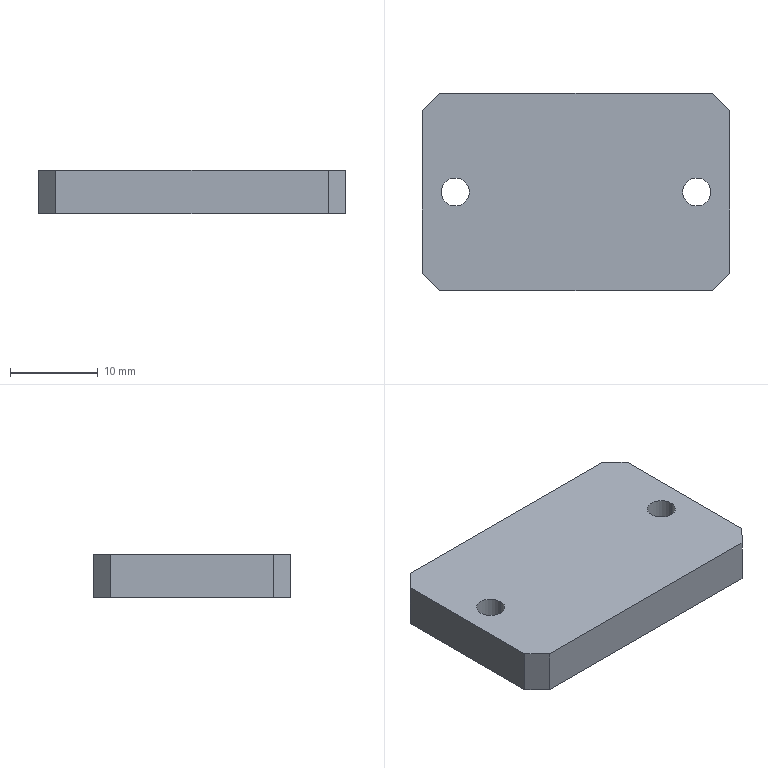Part | STEP file | PN_0031 | 1 solid | 14 faces | box 35 x 22.5 x 5 mm | volume 3817 mm3 | plane 10 | cylinder 4 | commonest cylinder face diameters 3.2 x4
STEP:
#1=CARTESIAN_POINT('',(0.,0.,0.));
#2=DIRECTION('',(0.,0.,1.));
#3=DIRECTION('',(1.,0.,0.));
#4=AXIS2_PLACEMENT_3D('',#1,#2,#3);
#5=CARTESIAN_POINT('',(-12.15,0.,0.));
#6=VERTEX_POINT('',#5);
#7=CARTESIAN_POINT('',(-12.15,0.,5.));
#8=VERTEX_POINT('',#7);
#9=CARTESIAN_POINT('',(-12.15,0.,5.));
#10=DIRECTION('',(0.,0.,1.));
#11=VECTOR('',#10,1.);
#12=LINE('',#9,#11);
#13=CARTESIAN_POINT('',(-13.75,0.,5.));
#14=DIRECTION('',(0.,0.,1.));
#15=DIRECTION('',(1.,0.,0.));
#16=AXIS2_PLACEMENT_3D('',#13,#14,#15);
#17=CYLINDRICAL_SURFACE('',#16,1.6);
#18=CARTESIAN_POINT('',(6.283,0.));
#19=DIRECTION('',(0.,1.));
#20=VECTOR('',#19,1.);
#21=LINE('',#18,#20);
#22=(GEOMETRIC_REPRESENTATION_CONTEXT(2)PARAMETRIC_REPRESENTATION_CONTEXT()REPRESENTATION_CONTEXT('',''));
#23=DEFINITIONAL_REPRESENTATION('',(#21),#22);
#24=PCURVE('',#17,#23);
#25=CARTESIAN_POINT('',(-13.75,0.,5.));
#26=DIRECTION('',(0.,0.,1.));
#27=DIRECTION('',(1.,0.,0.));
#28=AXIS2_PLACEMENT_3D('',#25,#26,#27);
#29=CYLINDRICAL_SURFACE('',#28,1.6);
#30=CARTESIAN_POINT('',(0.,0.));
#31=DIRECTION('',(0.,1.));
#32=VECTOR('',#31,1.);
#33=LINE('',#30,#32);
#34=(GEOMETRIC_REPRESENTATION_CONTEXT(2)PARAMETRIC_REPRESENTATION_CONTEXT()REPRESENTATION_CONTEXT('',''));
#35=DEFINITIONAL_REPRESENTATION('',(#33),#34);
#36=PCURVE('',#29,#35);
#37=SURFACE_CURVE('',#12,(#24,#36),.PCURVE_S1.);
#38=EDGE_CURVE('',#6,#8,#37,.T.);
#39=ORIENTED_EDGE('',*,*,#38,.T.);
#40=CARTESIAN_POINT('',(-15.35,0.,5.));
#41=VERTEX_POINT('',#40);
#42=CARTESIAN_POINT('',(-13.75,0.,5.));
#43=DIRECTION('',(0.,0.,1.));
#44=DIRECTION('',(1.,0.,0.));
#45=AXIS2_PLACEMENT_3D('',#42,#43,#44);
#46=CIRCLE('',#45,1.6);
#47=CARTESIAN_POINT('',(0.,0.));
#48=DIRECTION('',(1.,0.));
#49=VECTOR('',#48,1.);
#50=LINE('',#47,#49);
#51=(GEOMETRIC_REPRESENTATION_CONTEXT(2)PARAMETRIC_REPRESENTATION_CONTEXT()REPRESENTATION_CONTEXT('',''));
#52=DEFINITIONAL_REPRESENTATION('',(#50),#51);
#53=PCURVE('',#17,#52);
#54=CARTESIAN_POINT('',(0.,0.,5.));
#55=DIRECTION('',(0.,0.,1.));
#56=DIRECTION('',(1.,0.,0.));
#57=AXIS2_PLACEMENT_3D('',#54,#55,#56);
#58=PLANE('',#57);
#59=CARTESIAN_POINT('',(-13.75,0.));
#60=DIRECTION('',(1.,0.));
#61=AXIS2_PLACEMENT_2D('',#59,#60);
#62=CIRCLE('',#61,1.6);
#63=(GEOMETRIC_REPRESENTATION_CONTEXT(2)PARAMETRIC_REPRESENTATION_CONTEXT()REPRESENTATION_CONTEXT('',''));
#64=DEFINITIONAL_REPRESENTATION('',(#62),#63);
#65=PCURVE('',#58,#64);
#66=SURFACE_CURVE('',#46,(#53,#65),.PCURVE_S1.);
#67=EDGE_CURVE('',#41,#8,#66,.T.);
#68=ORIENTED_EDGE('',*,*,#67,.F.);
#69=CARTESIAN_POINT('',(-15.35,0.,0.));
#70=VERTEX_POINT('',#69);
#71=CARTESIAN_POINT('',(-15.35,0.,5.));
#72=DIRECTION('',(0.,0.,1.));
#73=VECTOR('',#72,1.);
#74=LINE('',#71,#73);
#75=CARTESIAN_POINT('',(3.142,0.));
#76=DIRECTION('',(0.,1.));
#77=VECTOR('',#76,1.);
#78=LINE('',#75,#77);
#79=(GEOMETRIC_REPRESENTATION_CONTEXT(2)PARAMETRIC_REPRESENTATION_CONTEXT()REPRESENTATION_CONTEXT('',''));
#80=DEFINITIONAL_REPRESENTATION('',(#78),#79);
#81=PCURVE('',#17,#80);
#82=CARTESIAN_POINT('',(3.142,0.));
#83=DIRECTION('',(0.,1.));
#84=VECTOR('',#83,1.);
#85=LINE('',#82,#84);
#86=(GEOMETRIC_REPRESENTATION_CONTEXT(2)PARAMETRIC_REPRESENTATION_CONTEXT()REPRESENTATION_CONTEXT('',''));
#87=DEFINITIONAL_REPRESENTATION('',(#85),#86);
#88=PCURVE('',#29,#87);
#89=SURFACE_CURVE('',#74,(#81,#88),.PCURVE_S1.);
#90=EDGE_CURVE('',#70,#41,#89,.T.);
#91=ORIENTED_EDGE('',*,*,#90,.F.);
#92=CARTESIAN_POINT('',(-13.75,0.,0.));
#93=DIRECTION('',(0.,0.,1.));
#94=DIRECTION('',(1.,0.,0.));
#95=AXIS2_PLACEMENT_3D('',#92,#93,#94);
#96=CIRCLE('',#95,1.6);
#97=CARTESIAN_POINT('',(0.,-5.));
#98=DIRECTION('',(1.,0.));
#99=VECTOR('',#98,1.);
#100=LINE('',#97,#99);
#101=(GEOMETRIC_REPRESENTATION_CONTEXT(2)PARAMETRIC_REPRESENTATION_CONTEXT()REPRESENTATION_CONTEXT('',''));
#102=DEFINITIONAL_REPRESENTATION('',(#100),#101);
#103=PCURVE('',#17,#102);
#104=CARTESIAN_POINT('',(0.,0.,0.));
#105=DIRECTION('',(0.,0.,1.));
#106=DIRECTION('',(1.,0.,0.));
#107=AXIS2_PLACEMENT_3D('',#104,#105,#106);
#108=PLANE('',#107);
#109=CARTESIAN_POINT('',(-13.75,0.));
#110=DIRECTION('',(1.,0.));
#111=AXIS2_PLACEMENT_2D('',#109,#110);
#112=CIRCLE('',#111,1.6);
#113=(GEOMETRIC_REPRESENTATION_CONTEXT(2)PARAMETRIC_REPRESENTATION_CONTEXT()REPRESENTATION_CONTEXT('',''));
#114=DEFINITIONAL_REPRESENTATION('',(#112),#113);
#115=PCURVE('',#108,#114);
#116=SURFACE_CURVE('',#96,(#103,#115),.PCURVE_S1.);
#117=EDGE_CURVE('',#70,#6,#116,.T.);
#118=ORIENTED_EDGE('',*,*,#117,.T.);
#119=EDGE_LOOP('',(#39,#68,#91,#118));
#120=FACE_BOUND('',#119,.F.);
#121=ADVANCED_FACE('',(#120),#17,.F.);
#122=CARTESIAN_POINT('',(15.35,0.,0.));
#123=VERTEX_POINT('',#122);
#124=CARTESIAN_POINT('',(15.35,0.,5.));
#125=VERTEX_POINT('',#124);
#126=CARTESIAN_POINT('',(15.35,0.,5.));
#127=DIRECTION('',(0.,0.,1.));
#128=VECTOR('',#127,1.);
#129=LINE('',#126,#128);
#130=CARTESIAN_POINT('',(13.75,0.,5.));
#131=DIRECTION('',(0.,0.,1.));
#132=DIRECTION('',(1.,0.,0.));
#133=AXIS2_PLACEMENT_3D('',#130,#131,#132);
#134=CYLINDRICAL_SURFACE('',#133,1.6);
#135=CARTESIAN_POINT('',(6.283,0.));
#136=DIRECTION('',(0.,1.));
#137=VECTOR('',#136,1.);
#138=LINE('',#135,#137);
#139=(GEOMETRIC_REPRESENTATION_CONTEXT(2)PARAMETRIC_REPRESENTATION_CONTEXT()REPRESENTATION_CONTEXT('',''));
#140=DEFINITIONAL_REPRESENTATION('',(#138),#139);
#141=PCURVE('',#134,#140);
#142=CARTESIAN_POINT('',(13.75,0.,5.));
#143=DIRECTION('',(0.,0.,1.));
#144=DIRECTION('',(1.,0.,0.));
#145=AXIS2_PLACEMENT_3D('',#142,#143,#144);
#146=CYLINDRICAL_SURFACE('',#145,1.6);
#147=CARTESIAN_POINT('',(0.,0.));
#148=DIRECTION('',(0.,1.));
#149=VECTOR('',#148,1.);
#150=LINE('',#147,#149);
#151=(GEOMETRIC_REPRESENTATION_CONTEXT(2)PARAMETRIC_REPRESENTATION_CONTEXT()REPRESENTATION_CONTEXT('',''));
#152=DEFINITIONAL_REPRESENTATION('',(#150),#151);
#153=PCURVE('',#146,#152);
#154=SURFACE_CURVE('',#129,(#141,#153),.PCURVE_S1.);
#155=EDGE_CURVE('',#123,#125,#154,.T.);
#156=ORIENTED_EDGE('',*,*,#155,.T.);
#157=CARTESIAN_POINT('',(12.15,0.,5.));
#158=VERTEX_POINT('',#157);
#159=CARTESIAN_POINT('',(13.75,0.,5.));
#160=DIRECTION('',(0.,0.,1.));
#161=DIRECTION('',(1.,0.,0.));
#162=AXIS2_PLACEMENT_3D('',#159,#160,#161);
#163=CIRCLE('',#162,1.6);
#164=CARTESIAN_POINT('',(0.,0.));
#165=DIRECTION('',(1.,0.));
#166=VECTOR('',#165,1.);
#167=LINE('',#164,#166);
#168=(GEOMETRIC_REPRESENTATION_CONTEXT(2)PARAMETRIC_REPRESENTATION_CONTEXT()REPRESENTATION_CONTEXT('',''));
#169=DEFINITIONAL_REPRESENTATION('',(#167),#168);
#170=PCURVE('',#134,#169);
#171=CARTESIAN_POINT('',(13.75,0.));
#172=DIRECTION('',(1.,0.));
#173=AXIS2_PLACEMENT_2D('',#171,#172);
#174=CIRCLE('',#173,1.6);
#175=(GEOMETRIC_REPRESENTATION_CONTEXT(2)PARAMETRIC_REPRESENTATION_CONTEXT()REPRESENTATION_CONTEXT('',''));
#176=DEFINITIONAL_REPRESENTATION('',(#174),#175);
#177=PCURVE('',#58,#176);
#178=SURFACE_CURVE('',#163,(#170,#177),.PCURVE_S1.);
#179=EDGE_CURVE('',#158,#125,#178,.T.);
#180=ORIENTED_EDGE('',*,*,#179,.F.);
#181=CARTESIAN_POINT('',(12.15,0.,0.));
#182=VERTEX_POINT('',#181);
#183=CARTESIAN_POINT('',(12.15,0.,5.));
#184=DIRECTION('',(0.,0.,1.));
#185=VECTOR('',#184,1.);
#186=LINE('',#183,#185);
#187=CARTESIAN_POINT('',(3.142,0.));
#188=DIRECTION('',(0.,1.));
#189=VECTOR('',#188,1.);
#190=LINE('',#187,#189);
#191=(GEOMETRIC_REPRESENTATION_CONTEXT(2)PARAMETRIC_REPRESENTATION_CONTEXT()REPRESENTATION_CONTEXT('',''));
#192=DEFINITIONAL_REPRESENTATION('',(#190),#191);
#193=PCURVE('',#134,#192);
#194=CARTESIAN_POINT('',(3.142,0.));
#195=DIRECTION('',(0.,1.));
#196=VECTOR('',#195,1.);
#197=LINE('',#194,#196);
#198=(GEOMETRIC_REPRESENTATION_CONTEXT(2)PARAMETRIC_REPRESENTATION_CONTEXT()REPRESENTATION_CONTEXT('',''));
#199=DEFINITIONAL_REPRESENTATION('',(#197),#198);
#200=PCURVE('',#146,#199);
#201=SURFACE_CURVE('',#186,(#193,#200),.PCURVE_S1.);
#202=EDGE_CURVE('',#182,#158,#201,.T.);
#203=ORIENTED_EDGE('',*,*,#202,.F.);
#204=CARTESIAN_POINT('',(13.75,0.,0.));
#205=DIRECTION('',(0.,0.,1.));
#206=DIRECTION('',(1.,0.,0.));
#207=AXIS2_PLACEMENT_3D('',#204,#205,#206);
#208=CIRCLE('',#207,1.6);
#209=CARTESIAN_POINT('',(0.,-5.));
#210=DIRECTION('',(1.,0.));
#211=VECTOR('',#210,1.);
#212=LINE('',#209,#211);
#213=(GEOMETRIC_REPRESENTATION_CONTEXT(2)PARAMETRIC_REPRESENTATION_CONTEXT()REPRESENTATION_CONTEXT('',''));
#214=DEFINITIONAL_REPRESENTATION('',(#212),#213);
#215=PCURVE('',#134,#214);
#216=CARTESIAN_POINT('',(13.75,0.));
#217=DIRECTION('',(1.,0.));
#218=AXIS2_PLACEMENT_2D('',#216,#217);
#219=CIRCLE('',#218,1.6);
#220=(GEOMETRIC_REPRESENTATION_CONTEXT(2)PARAMETRIC_REPRESENTATION_CONTEXT()REPRESENTATION_CONTEXT('',''));
#221=DEFINITIONAL_REPRESENTATION('',(#219),#220);
#222=PCURVE('',#108,#221);
#223=SURFACE_CURVE('',#208,(#215,#222),.PCURVE_S1.);
#224=EDGE_CURVE('',#182,#123,#223,.T.);
#225=ORIENTED_EDGE('',*,*,#224,.T.);
#226=EDGE_LOOP('',(#156,#180,#203,#225));
#227=FACE_BOUND('',#226,.F.);
#228=ADVANCED_FACE('',(#227),#134,.F.);
#229=CARTESIAN_POINT('',(17.5,-9.25,5.));
#230=VERTEX_POINT('',#229);
#231=CARTESIAN_POINT('',(17.5,9.25,5.));
#232=VERTEX_POINT('',#231);
#233=CARTESIAN_POINT('',(17.5,11.25,5.));
#234=DIRECTION('',(0.,1.,0.));
#235=VECTOR('',#234,1.);
#236=LINE('',#233,#235);
#237=CARTESIAN_POINT('',(17.5,11.25,5.));
#238=DIRECTION('',(-1.,0.,0.));
#239=DIRECTION('',(0.,-1.,0.));
#240=AXIS2_PLACEMENT_3D('',#237,#238,#239);
#241=PLANE('',#240);
#242=CARTESIAN_POINT('',(0.,0.));
#243=DIRECTION('',(-1.,0.));
#244=VECTOR('',#243,1.);
#245=LINE('',#242,#244);
#246=(GEOMETRIC_REPRESENTATION_CONTEXT(2)PARAMETRIC_REPRESENTATION_CONTEXT()REPRESENTATION_CONTEXT('',''));
#247=DEFINITIONAL_REPRESENTATION('',(#245),#246);
#248=PCURVE('',#241,#247);
#249=CARTESIAN_POINT('',(17.5,11.25));
#250=DIRECTION('',(0.,1.));
#251=VECTOR('',#250,1.);
#252=LINE('',#249,#251);
#253=(GEOMETRIC_REPRESENTATION_CONTEXT(2)PARAMETRIC_REPRESENTATION_CONTEXT()REPRESENTATION_CONTEXT('',''));
#254=DEFINITIONAL_REPRESENTATION('',(#252),#253);
#255=PCURVE('',#58,#254);
#256=SURFACE_CURVE('',#236,(#248,#255),.PCURVE_S1.);
#257=EDGE_CURVE('',#230,#232,#256,.T.);
#258=ORIENTED_EDGE('',*,*,#257,.F.);
#259=CARTESIAN_POINT('',(17.5,-9.25,0.));
#260=VERTEX_POINT('',#259);
#261=CARTESIAN_POINT('',(17.5,-9.25,5.));
#262=DIRECTION('',(0.,0.,-1.));
#263=VECTOR('',#262,1.);
#264=LINE('',#261,#263);
#265=CARTESIAN_POINT('',(20.5,0.));
#266=DIRECTION('',(0.,-1.));
#267=VECTOR('',#266,1.);
#268=LINE('',#265,#267);
#269=(GEOMETRIC_REPRESENTATION_CONTEXT(2)PARAMETRIC_REPRESENTATION_CONTEXT()REPRESENTATION_CONTEXT('',''));
#270=DEFINITIONAL_REPRESENTATION('',(#268),#269);
#271=PCURVE('',#241,#270);
#272=CARTESIAN_POINT('',(17.5,-9.25,5.));
#273=DIRECTION('',(-0.7071,0.7071,0.));
#274=DIRECTION('',(0.,0.,-1.));
#275=AXIS2_PLACEMENT_3D('',#272,#273,#274);
#276=PLANE('',#275);
#277=CARTESIAN_POINT('',(0.,0.));
#278=DIRECTION('',(1.,0.));
#279=VECTOR('',#278,1.);
#280=LINE('',#277,#279);
#281=(GEOMETRIC_REPRESENTATION_CONTEXT(2)PARAMETRIC_REPRESENTATION_CONTEXT()REPRESENTATION_CONTEXT('',''));
#282=DEFINITIONAL_REPRESENTATION('',(#280),#281);
#283=PCURVE('',#276,#282);
#284=SURFACE_CURVE('',#264,(#271,#283),.PCURVE_S1.);
#285=EDGE_CURVE('',#230,#260,#284,.T.);
#286=ORIENTED_EDGE('',*,*,#285,.T.);
#287=CARTESIAN_POINT('',(17.5,9.25,0.));
#288=VERTEX_POINT('',#287);
#289=CARTESIAN_POINT('',(17.5,11.25,0.));
#290=DIRECTION('',(0.,1.,0.));
#291=VECTOR('',#290,1.);
#292=LINE('',#289,#291);
#293=CARTESIAN_POINT('',(0.,-5.));
#294=DIRECTION('',(-1.,0.));
#295=VECTOR('',#294,1.);
#296=LINE('',#293,#295);
#297=(GEOMETRIC_REPRESENTATION_CONTEXT(2)PARAMETRIC_REPRESENTATION_CONTEXT()REPRESENTATION_CONTEXT('',''));
#298=DEFINITIONAL_REPRESENTATION('',(#296),#297);
#299=PCURVE('',#241,#298);
#300=CARTESIAN_POINT('',(17.5,11.25));
#301=DIRECTION('',(0.,1.));
#302=VECTOR('',#301,1.);
#303=LINE('',#300,#302);
#304=(GEOMETRIC_REPRESENTATION_CONTEXT(2)PARAMETRIC_REPRESENTATION_CONTEXT()REPRESENTATION_CONTEXT('',''));
#305=DEFINITIONAL_REPRESENTATION('',(#303),#304);
#306=PCURVE('',#108,#305);
#307=SURFACE_CURVE('',#292,(#299,#306),.PCURVE_S1.);
#308=EDGE_CURVE('',#260,#288,#307,.T.);
#309=ORIENTED_EDGE('',*,*,#308,.T.);
#310=CARTESIAN_POINT('',(17.5,9.25,5.));
#311=DIRECTION('',(0.,0.,1.));
#312=VECTOR('',#311,1.);
#313=LINE('',#310,#312);
#314=CARTESIAN_POINT('',(2.,0.));
#315=DIRECTION('',(0.,1.));
#316=VECTOR('',#315,1.);
#317=LINE('',#314,#316);
#318=(GEOMETRIC_REPRESENTATION_CONTEXT(2)PARAMETRIC_REPRESENTATION_CONTEXT()REPRESENTATION_CONTEXT('',''));
#319=DEFINITIONAL_REPRESENTATION('',(#317),#318);
#320=PCURVE('',#241,#319);
#321=CARTESIAN_POINT('',(15.5,11.25,5.));
#322=DIRECTION('',(-0.7071,-0.7071,0.));
#323=DIRECTION('',(0.,0.,-1.));
#324=AXIS2_PLACEMENT_3D('',#321,#322,#323);
#325=PLANE('',#324);
#326=CARTESIAN_POINT('',(0.,2.828));
#327=DIRECTION('',(-1.,0.));
#328=VECTOR('',#327,1.);
#329=LINE('',#326,#328);
#330=(GEOMETRIC_REPRESENTATION_CONTEXT(2)PARAMETRIC_REPRESENTATION_CONTEXT()REPRESENTATION_CONTEXT('',''));
#331=DEFINITIONAL_REPRESENTATION('',(#329),#330);
#332=PCURVE('',#325,#331);
#333=SURFACE_CURVE('',#313,(#320,#332),.PCURVE_S1.);
#334=EDGE_CURVE('',#288,#232,#333,.T.);
#335=ORIENTED_EDGE('',*,*,#334,.T.);
#336=EDGE_LOOP('',(#258,#286,#309,#335));
#337=FACE_BOUND('',#336,.T.);
#338=ADVANCED_FACE('',(#337),#241,.F.);
#339=CARTESIAN_POINT('',(15.5,11.25,0.));
#340=VERTEX_POINT('',#339);
#341=CARTESIAN_POINT('',(-15.5,11.25,0.));
#342=VERTEX_POINT('',#341);
#343=CARTESIAN_POINT('',(-17.5,11.25,0.));
#344=DIRECTION('',(-1.,0.,0.));
#345=VECTOR('',#344,1.);
#346=LINE('',#343,#345);
#347=CARTESIAN_POINT('',(-17.5,11.25,5.));
#348=DIRECTION('',(0.,-1.,0.));
#349=DIRECTION('',(1.,0.,0.));
#350=AXIS2_PLACEMENT_3D('',#347,#348,#349);
#351=PLANE('',#350);
#352=CARTESIAN_POINT('',(0.,-5.));
#353=DIRECTION('',(-1.,0.));
#354=VECTOR('',#353,1.);
#355=LINE('',#352,#354);
#356=(GEOMETRIC_REPRESENTATION_CONTEXT(2)PARAMETRIC_REPRESENTATION_CONTEXT()REPRESENTATION_CONTEXT('',''));
#357=DEFINITIONAL_REPRESENTATION('',(#355),#356);
#358=PCURVE('',#351,#357);
#359=CARTESIAN_POINT('',(-17.5,11.25));
#360=DIRECTION('',(-1.,0.));
#361=VECTOR('',#360,1.);
#362=LINE('',#359,#361);
#363=(GEOMETRIC_REPRESENTATION_CONTEXT(2)PARAMETRIC_REPRESENTATION_CONTEXT()REPRESENTATION_CONTEXT('',''));
#364=DEFINITIONAL_REPRESENTATION('',(#362),#363);
#365=PCURVE('',#108,#364);
#366=SURFACE_CURVE('',#346,(#358,#365),.PCURVE_S1.);
#367=EDGE_CURVE('',#340,#342,#366,.T.);
#368=ORIENTED_EDGE('',*,*,#367,.T.);
#369=CARTESIAN_POINT('',(-15.5,11.25,5.));
#370=VERTEX_POINT('',#369);
#371=CARTESIAN_POINT('',(-15.5,11.25,5.));
#372=DIRECTION('',(0.,0.,1.));
#373=VECTOR('',#372,1.);
#374=LINE('',#371,#373);
#375=CARTESIAN_POINT('',(2.,0.));
#376=DIRECTION('',(0.,1.));
#377=VECTOR('',#376,1.);
#378=LINE('',#375,#377);
#379=(GEOMETRIC_REPRESENTATION_CONTEXT(2)PARAMETRIC_REPRESENTATION_CONTEXT()REPRESENTATION_CONTEXT('',''));
#380=DEFINITIONAL_REPRESENTATION('',(#378),#379);
#381=PCURVE('',#351,#380);
#382=CARTESIAN_POINT('',(-17.5,9.25,5.));
#383=DIRECTION('',(0.7071,-0.7071,0.));
#384=DIRECTION('',(0.,0.,-1.));
#385=AXIS2_PLACEMENT_3D('',#382,#383,#384);
#386=PLANE('',#385);
#387=CARTESIAN_POINT('',(0.,2.828));
#388=DIRECTION('',(-1.,0.));
#389=VECTOR('',#388,1.);
#390=LINE('',#387,#389);
#391=(GEOMETRIC_REPRESENTATION_CONTEXT(2)PARAMETRIC_REPRESENTATION_CONTEXT()REPRESENTATION_CONTEXT('',''));
#392=DEFINITIONAL_REPRESENTATION('',(#390),#391);
#393=PCURVE('',#386,#392);
#394=SURFACE_CURVE('',#374,(#381,#393),.PCURVE_S1.);
#395=EDGE_CURVE('',#342,#370,#394,.T.);
#396=ORIENTED_EDGE('',*,*,#395,.T.);
#397=CARTESIAN_POINT('',(15.5,11.25,5.));
#398=VERTEX_POINT('',#397);
#399=CARTESIAN_POINT('',(-17.5,11.25,5.));
#400=DIRECTION('',(-1.,0.,0.));
#401=VECTOR('',#400,1.);
#402=LINE('',#399,#401);
#403=CARTESIAN_POINT('',(0.,0.));
#404=DIRECTION('',(-1.,0.));
#405=VECTOR('',#404,1.);
#406=LINE('',#403,#405);
#407=(GEOMETRIC_REPRESENTATION_CONTEXT(2)PARAMETRIC_REPRESENTATION_CONTEXT()REPRESENTATION_CONTEXT('',''));
#408=DEFINITIONAL_REPRESENTATION('',(#406),#407);
#409=PCURVE('',#351,#408);
#410=CARTESIAN_POINT('',(-17.5,11.25));
#411=DIRECTION('',(-1.,0.));
#412=VECTOR('',#411,1.);
#413=LINE('',#410,#412);
#414=(GEOMETRIC_REPRESENTATION_CONTEXT(2)PARAMETRIC_REPRESENTATION_CONTEXT()REPRESENTATION_CONTEXT('',''));
#415=DEFINITIONAL_REPRESENTATION('',(#413),#414);
#416=PCURVE('',#58,#415);
#417=SURFACE_CURVE('',#402,(#409,#416),.PCURVE_S1.);
#418=EDGE_CURVE('',#398,#370,#417,.T.);
#419=ORIENTED_EDGE('',*,*,#418,.F.);
#420=CARTESIAN_POINT('',(15.5,11.25,5.));
#421=DIRECTION('',(0.,0.,-1.));
#422=VECTOR('',#421,1.);
#423=LINE('',#420,#422);
#424=CARTESIAN_POINT('',(33.,0.));
#425=DIRECTION('',(0.,-1.));
#426=VECTOR('',#425,1.);
#427=LINE('',#424,#426);
#428=(GEOMETRIC_REPRESENTATION_CONTEXT(2)PARAMETRIC_REPRESENTATION_CONTEXT()REPRESENTATION_CONTEXT('',''));
#429=DEFINITIONAL_REPRESENTATION('',(#427),#428);
#430=PCURVE('',#351,#429);
#431=CARTESIAN_POINT('',(0.,0.));
#432=DIRECTION('',(1.,0.));
#433=VECTOR('',#432,1.);
#434=LINE('',#431,#433);
#435=(GEOMETRIC_REPRESENTATION_CONTEXT(2)PARAMETRIC_REPRESENTATION_CONTEXT()REPRESENTATION_CONTEXT('',''));
#436=DEFINITIONAL_REPRESENTATION('',(#434),#435);
#437=PCURVE('',#325,#436);
#438=SURFACE_CURVE('',#423,(#430,#437),.PCURVE_S1.);
#439=EDGE_CURVE('',#398,#340,#438,.T.);
#440=ORIENTED_EDGE('',*,*,#439,.T.);
#441=EDGE_LOOP('',(#368,#396,#419,#440));
#442=FACE_BOUND('',#441,.T.);
#443=ADVANCED_FACE('',(#442),#351,.F.);
#444=CARTESIAN_POINT('',(-17.5,9.25,5.));
#445=VERTEX_POINT('',#444);
#446=CARTESIAN_POINT('',(-17.5,-9.25,5.));
#447=VERTEX_POINT('',#446);
#448=CARTESIAN_POINT('',(-17.5,11.25,5.));
#449=DIRECTION('',(0.,-1.,0.));
#450=VECTOR('',#449,1.);
#451=LINE('',#448,#450);
#452=CARTESIAN_POINT('',(-17.5,11.25,5.));
#453=DIRECTION('',(1.,0.,0.));
#454=DIRECTION('',(0.,0.,-1.));
#455=AXIS2_PLACEMENT_3D('',#452,#453,#454);
#456=PLANE('',#455);
#457=CARTESIAN_POINT('',(0.,0.));
#458=DIRECTION('',(0.,-1.));
#459=VECTOR('',#458,1.);
#460=LINE('',#457,#459);
#461=(GEOMETRIC_REPRESENTATION_CONTEXT(2)PARAMETRIC_REPRESENTATION_CONTEXT()REPRESENTATION_CONTEXT('',''));
#462=DEFINITIONAL_REPRESENTATION('',(#460),#461);
#463=PCURVE('',#456,#462);
#464=CARTESIAN_POINT('',(-17.5,11.25));
#465=DIRECTION('',(0.,-1.));
#466=VECTOR('',#465,1.);
#467=LINE('',#464,#466);
#468=(GEOMETRIC_REPRESENTATION_CONTEXT(2)PARAMETRIC_REPRESENTATION_CONTEXT()REPRESENTATION_CONTEXT('',''));
#469=DEFINITIONAL_REPRESENTATION('',(#467),#468);
#470=PCURVE('',#58,#469);
#471=SURFACE_CURVE('',#451,(#463,#470),.PCURVE_S1.);
#472=EDGE_CURVE('',#445,#447,#471,.T.);
#473=ORIENTED_EDGE('',*,*,#472,.F.);
#474=CARTESIAN_POINT('',(-17.5,9.25,0.));
#475=VERTEX_POINT('',#474);
#476=CARTESIAN_POINT('',(-17.5,9.25,5.));
#477=DIRECTION('',(0.,0.,-1.));
#478=VECTOR('',#477,1.);
#479=LINE('',#476,#478);
#480=CARTESIAN_POINT('',(0.,-2.));
#481=DIRECTION('',(1.,0.));
#482=VECTOR('',#481,1.);
#483=LINE('',#480,#482);
#484=(GEOMETRIC_REPRESENTATION_CONTEXT(2)PARAMETRIC_REPRESENTATION_CONTEXT()REPRESENTATION_CONTEXT('',''));
#485=DEFINITIONAL_REPRESENTATION('',(#483),#484);
#486=PCURVE('',#456,#485);
#487=CARTESIAN_POINT('',(0.,0.));
#488=DIRECTION('',(1.,0.));
#489=VECTOR('',#488,1.);
#490=LINE('',#487,#489);
#491=(GEOMETRIC_REPRESENTATION_CONTEXT(2)PARAMETRIC_REPRESENTATION_CONTEXT()REPRESENTATION_CONTEXT('',''));
#492=DEFINITIONAL_REPRESENTATION('',(#490),#491);
#493=PCURVE('',#386,#492);
#494=SURFACE_CURVE('',#479,(#486,#493),.PCURVE_S1.);
#495=EDGE_CURVE('',#445,#475,#494,.T.);
#496=ORIENTED_EDGE('',*,*,#495,.T.);
#497=CARTESIAN_POINT('',(-17.5,-9.25,0.));
#498=VERTEX_POINT('',#497);
#499=CARTESIAN_POINT('',(-17.5,11.25,0.));
#500=DIRECTION('',(0.,-1.,0.));
#501=VECTOR('',#500,1.);
#502=LINE('',#499,#501);
#503=CARTESIAN_POINT('',(5.,0.));
#504=DIRECTION('',(0.,-1.));
#505=VECTOR('',#504,1.);
#506=LINE('',#503,#505);
#507=(GEOMETRIC_REPRESENTATION_CONTEXT(2)PARAMETRIC_REPRESENTATION_CONTEXT()REPRESENTATION_CONTEXT('',''));
#508=DEFINITIONAL_REPRESENTATION('',(#506),#507);
#509=PCURVE('',#456,#508);
#510=CARTESIAN_POINT('',(-17.5,11.25));
#511=DIRECTION('',(0.,-1.));
#512=VECTOR('',#511,1.);
#513=LINE('',#510,#512);
#514=(GEOMETRIC_REPRESENTATION_CONTEXT(2)PARAMETRIC_REPRESENTATION_CONTEXT()REPRESENTATION_CONTEXT('',''));
#515=DEFINITIONAL_REPRESENTATION('',(#513),#514);
#516=PCURVE('',#108,#515);
#517=SURFACE_CURVE('',#502,(#509,#516),.PCURVE_S1.);
#518=EDGE_CURVE('',#475,#498,#517,.T.);
#519=ORIENTED_EDGE('',*,*,#518,.T.);
#520=CARTESIAN_POINT('',(-17.5,-9.25,5.));
#521=DIRECTION('',(0.,0.,1.));
#522=VECTOR('',#521,1.);
#523=LINE('',#520,#522);
#524=CARTESIAN_POINT('',(0.,-20.5));
#525=DIRECTION('',(-1.,0.));
#526=VECTOR('',#525,1.);
#527=LINE('',#524,#526);
#528=(GEOMETRIC_REPRESENTATION_CONTEXT(2)PARAMETRIC_REPRESENTATION_CONTEXT()REPRESENTATION_CONTEXT('',''));
#529=DEFINITIONAL_REPRESENTATION('',(#527),#528);
#530=PCURVE('',#456,#529);
#531=CARTESIAN_POINT('',(-15.5,-11.25,5.));
#532=DIRECTION('',(0.7071,0.7071,0.));
#533=DIRECTION('',(0.,0.,-1.));
#534=AXIS2_PLACEMENT_3D('',#531,#532,#533);
#535=PLANE('',#534);
#536=CARTESIAN_POINT('',(0.,2.828));
#537=DIRECTION('',(-1.,0.));
#538=VECTOR('',#537,1.);
#539=LINE('',#536,#538);
#540=(GEOMETRIC_REPRESENTATION_CONTEXT(2)PARAMETRIC_REPRESENTATION_CONTEXT()REPRESENTATION_CONTEXT('',''));
#541=DEFINITIONAL_REPRESENTATION('',(#539),#540);
#542=PCURVE('',#535,#541);
#543=SURFACE_CURVE('',#523,(#530,#542),.PCURVE_S1.);
#544=EDGE_CURVE('',#498,#447,#543,.T.);
#545=ORIENTED_EDGE('',*,*,#544,.T.);
#546=EDGE_LOOP('',(#473,#496,#519,#545));
#547=FACE_BOUND('',#546,.T.);
#548=ADVANCED_FACE('',(#547),#456,.F.);
#549=CARTESIAN_POINT('',(-15.5,-11.25,5.));
#550=VERTEX_POINT('',#549);
#551=CARTESIAN_POINT('',(15.5,-11.25,5.));
#552=VERTEX_POINT('',#551);
#553=CARTESIAN_POINT('',(-17.5,-11.25,5.));
#554=DIRECTION('',(1.,0.,0.));
#555=VECTOR('',#554,1.);
#556=LINE('',#553,#555);
#557=CARTESIAN_POINT('',(-17.5,-11.25,5.));
#558=DIRECTION('',(0.,1.,0.));
#559=DIRECTION('',(0.,0.,1.));
#560=AXIS2_PLACEMENT_3D('',#557,#558,#559);
#561=PLANE('',#560);
#562=CARTESIAN_POINT('',(0.,0.));
#563=DIRECTION('',(0.,1.));
#564=VECTOR('',#563,1.);
#565=LINE('',#562,#564);
#566=(GEOMETRIC_REPRESENTATION_CONTEXT(2)PARAMETRIC_REPRESENTATION_CONTEXT()REPRESENTATION_CONTEXT('',''));
#567=DEFINITIONAL_REPRESENTATION('',(#565),#566);
#568=PCURVE('',#561,#567);
#569=CARTESIAN_POINT('',(-17.5,-11.25));
#570=DIRECTION('',(1.,0.));
#571=VECTOR('',#570,1.);
#572=LINE('',#569,#571);
#573=(GEOMETRIC_REPRESENTATION_CONTEXT(2)PARAMETRIC_REPRESENTATION_CONTEXT()REPRESENTATION_CONTEXT('',''));
#574=DEFINITIONAL_REPRESENTATION('',(#572),#573);
#575=PCURVE('',#58,#574);
#576=SURFACE_CURVE('',#556,(#568,#575),.PCURVE_S1.);
#577=EDGE_CURVE('',#550,#552,#576,.T.);
#578=ORIENTED_EDGE('',*,*,#577,.F.);
#579=CARTESIAN_POINT('',(-15.5,-11.25,0.));
#580=VERTEX_POINT('',#579);
#581=CARTESIAN_POINT('',(-15.5,-11.25,5.));
#582=DIRECTION('',(0.,0.,-1.));
#583=VECTOR('',#582,1.);
#584=LINE('',#581,#583);
#585=CARTESIAN_POINT('',(0.,2.));
#586=DIRECTION('',(-1.,0.));
#587=VECTOR('',#586,1.);
#588=LINE('',#585,#587);
#589=(GEOMETRIC_REPRESENTATION_CONTEXT(2)PARAMETRIC_REPRESENTATION_CONTEXT()REPRESENTATION_CONTEXT('',''));
#590=DEFINITIONAL_REPRESENTATION('',(#588),#589);
#591=PCURVE('',#561,#590);
#592=CARTESIAN_POINT('',(0.,0.));
#593=DIRECTION('',(1.,0.));
#594=VECTOR('',#593,1.);
#595=LINE('',#592,#594);
#596=(GEOMETRIC_REPRESENTATION_CONTEXT(2)PARAMETRIC_REPRESENTATION_CONTEXT()REPRESENTATION_CONTEXT('',''));
#597=DEFINITIONAL_REPRESENTATION('',(#595),#596);
#598=PCURVE('',#535,#597);
#599=SURFACE_CURVE('',#584,(#591,#598),.PCURVE_S1.);
#600=EDGE_CURVE('',#550,#580,#599,.T.);
#601=ORIENTED_EDGE('',*,*,#600,.T.);
#602=CARTESIAN_POINT('',(15.5,-11.25,0.));
#603=VERTEX_POINT('',#602);
#604=CARTESIAN_POINT('',(-17.5,-11.25,0.));
#605=DIRECTION('',(1.,0.,0.));
#606=VECTOR('',#605,1.);
#607=LINE('',#604,#606);
#608=CARTESIAN_POINT('',(-5.,0.));
#609=DIRECTION('',(0.,1.));
#610=VECTOR('',#609,1.);
#611=LINE('',#608,#610);
#612=(GEOMETRIC_REPRESENTATION_CONTEXT(2)PARAMETRIC_REPRESENTATION_CONTEXT()REPRESENTATION_CONTEXT('',''));
#613=DEFINITIONAL_REPRESENTATION('',(#611),#612);
#614=PCURVE('',#561,#613);
#615=CARTESIAN_POINT('',(-17.5,-11.25));
#616=DIRECTION('',(1.,0.));
#617=VECTOR('',#616,1.);
#618=LINE('',#615,#617);
#619=(GEOMETRIC_REPRESENTATION_CONTEXT(2)PARAMETRIC_REPRESENTATION_CONTEXT()REPRESENTATION_CONTEXT('',''));
#620=DEFINITIONAL_REPRESENTATION('',(#618),#619);
#621=PCURVE('',#108,#620);
#622=SURFACE_CURVE('',#607,(#614,#621),.PCURVE_S1.);
#623=EDGE_CURVE('',#580,#603,#622,.T.);
#624=ORIENTED_EDGE('',*,*,#623,.T.);
#625=CARTESIAN_POINT('',(15.5,-11.25,5.));
#626=DIRECTION('',(0.,0.,1.));
#627=VECTOR('',#626,1.);
#628=LINE('',#625,#627);
#629=CARTESIAN_POINT('',(0.,33.));
#630=DIRECTION('',(1.,0.));
#631=VECTOR('',#630,1.);
#632=LINE('',#629,#631);
#633=(GEOMETRIC_REPRESENTATION_CONTEXT(2)PARAMETRIC_REPRESENTATION_CONTEXT()REPRESENTATION_CONTEXT('',''));
#634=DEFINITIONAL_REPRESENTATION('',(#632),#633);
#635=PCURVE('',#561,#634);
#636=CARTESIAN_POINT('',(0.,2.828));
#637=DIRECTION('',(-1.,0.));
#638=VECTOR('',#637,1.);
#639=LINE('',#636,#638);
#640=(GEOMETRIC_REPRESENTATION_CONTEXT(2)PARAMETRIC_REPRESENTATION_CONTEXT()REPRESENTATION_CONTEXT('',''));
#641=DEFINITIONAL_REPRESENTATION('',(#639),#640);
#642=PCURVE('',#276,#641);
#643=SURFACE_CURVE('',#628,(#635,#642),.PCURVE_S1.);
#644=EDGE_CURVE('',#603,#552,#643,.T.);
#645=ORIENTED_EDGE('',*,*,#644,.T.);
#646=EDGE_LOOP('',(#578,#601,#624,#645));
#647=FACE_BOUND('',#646,.T.);
#648=ADVANCED_FACE('',(#647),#561,.F.);
#649=CARTESIAN_POINT('',(-13.75,0.,5.));
#650=DIRECTION('',(0.,0.,1.));
#651=DIRECTION('',(1.,0.,0.));
#652=AXIS2_PLACEMENT_3D('',#649,#650,#651);
#653=CIRCLE('',#652,1.6);
#654=CARTESIAN_POINT('',(-13.75,0.));
#655=DIRECTION('',(1.,0.));
#656=AXIS2_PLACEMENT_2D('',#654,#655);
#657=CIRCLE('',#656,1.6);
#658=(GEOMETRIC_REPRESENTATION_CONTEXT(2)PARAMETRIC_REPRESENTATION_CONTEXT()REPRESENTATION_CONTEXT('',''));
#659=DEFINITIONAL_REPRESENTATION('',(#657),#658);
#660=PCURVE('',#58,#659);
#661=CARTESIAN_POINT('',(0.,0.));
#662=DIRECTION('',(1.,0.));
#663=VECTOR('',#662,1.);
#664=LINE('',#661,#663);
#665=(GEOMETRIC_REPRESENTATION_CONTEXT(2)PARAMETRIC_REPRESENTATION_CONTEXT()REPRESENTATION_CONTEXT('',''));
#666=DEFINITIONAL_REPRESENTATION('',(#664),#665);
#667=PCURVE('',#29,#666);
#668=SURFACE_CURVE('',#653,(#660,#667),.PCURVE_S1.);
#669=EDGE_CURVE('',#8,#41,#668,.T.);
#670=ORIENTED_EDGE('',*,*,#669,.F.);
#671=ORIENTED_EDGE('',*,*,#67,.F.);
#672=EDGE_LOOP('',(#670,#671));
#673=FACE_BOUND('',#672,.T.);
#674=CARTESIAN_POINT('',(13.75,0.,5.));
#675=DIRECTION('',(0.,0.,1.));
#676=DIRECTION('',(1.,0.,0.));
#677=AXIS2_PLACEMENT_3D('',#674,#675,#676);
#678=CIRCLE('',#677,1.6);
#679=CARTESIAN_POINT('',(13.75,0.));
#680=DIRECTION('',(1.,0.));
#681=AXIS2_PLACEMENT_2D('',#679,#680);
#682=CIRCLE('',#681,1.6);
#683=(GEOMETRIC_REPRESENTATION_CONTEXT(2)PARAMETRIC_REPRESENTATION_CONTEXT()REPRESENTATION_CONTEXT('',''));
#684=DEFINITIONAL_REPRESENTATION('',(#682),#683);
#685=PCURVE('',#58,#684);
#686=CARTESIAN_POINT('',(0.,0.));
#687=DIRECTION('',(1.,0.));
#688=VECTOR('',#687,1.);
#689=LINE('',#686,#688);
#690=(GEOMETRIC_REPRESENTATION_CONTEXT(2)PARAMETRIC_REPRESENTATION_CONTEXT()REPRESENTATION_CONTEXT('',''));
#691=DEFINITIONAL_REPRESENTATION('',(#689),#690);
#692=PCURVE('',#146,#691);
#693=SURFACE_CURVE('',#678,(#685,#692),.PCURVE_S1.);
#694=EDGE_CURVE('',#125,#158,#693,.T.);
#695=ORIENTED_EDGE('',*,*,#694,.F.);
#696=ORIENTED_EDGE('',*,*,#179,.F.);
#697=EDGE_LOOP('',(#695,#696));
#698=FACE_BOUND('',#697,.T.);
#699=ORIENTED_EDGE('',*,*,#418,.T.);
#700=CARTESIAN_POINT('',(-13.375,13.375,5.));
#701=DIRECTION('',(-0.7071,-0.7071,0.));
#702=VECTOR('',#701,1.);
#703=LINE('',#700,#702);
#704=CARTESIAN_POINT('',(-13.375,13.375));
#705=DIRECTION('',(-0.7071,-0.7071));
#706=VECTOR('',#705,1.);
#707=LINE('',#704,#706);
#708=(GEOMETRIC_REPRESENTATION_CONTEXT(2)PARAMETRIC_REPRESENTATION_CONTEXT()REPRESENTATION_CONTEXT('',''));
#709=DEFINITIONAL_REPRESENTATION('',(#707),#708);
#710=PCURVE('',#58,#709);
#711=CARTESIAN_POINT('',(0.,5.834));
#712=DIRECTION('',(0.,-1.));
#713=VECTOR('',#712,1.);
#714=LINE('',#711,#713);
#715=(GEOMETRIC_REPRESENTATION_CONTEXT(2)PARAMETRIC_REPRESENTATION_CONTEXT()REPRESENTATION_CONTEXT('',''));
#716=DEFINITIONAL_REPRESENTATION('',(#714),#715);
#717=PCURVE('',#386,#716);
#718=SURFACE_CURVE('',#703,(#710,#717),.PCURVE_S1.);
#719=EDGE_CURVE('',#370,#445,#718,.T.);
#720=ORIENTED_EDGE('',*,*,#719,.T.);
#721=ORIENTED_EDGE('',*,*,#472,.T.);
#722=CARTESIAN_POINT('',(-13.375,-13.375,5.));
#723=DIRECTION('',(0.7071,-0.7071,0.));
#724=VECTOR('',#723,1.);
#725=LINE('',#722,#724);
#726=CARTESIAN_POINT('',(-13.375,-13.375));
#727=DIRECTION('',(0.7071,-0.7071));
#728=VECTOR('',#727,1.);
#729=LINE('',#726,#728);
#730=(GEOMETRIC_REPRESENTATION_CONTEXT(2)PARAMETRIC_REPRESENTATION_CONTEXT()REPRESENTATION_CONTEXT('',''));
#731=DEFINITIONAL_REPRESENTATION('',(#729),#730);
#732=PCURVE('',#58,#731);
#733=CARTESIAN_POINT('',(0.,-3.005));
#734=DIRECTION('',(0.,-1.));
#735=VECTOR('',#734,1.);
#736=LINE('',#733,#735);
#737=(GEOMETRIC_REPRESENTATION_CONTEXT(2)PARAMETRIC_REPRESENTATION_CONTEXT()REPRESENTATION_CONTEXT('',''));
#738=DEFINITIONAL_REPRESENTATION('',(#736),#737);
#739=PCURVE('',#535,#738);
#740=SURFACE_CURVE('',#725,(#732,#739),.PCURVE_S1.);
#741=EDGE_CURVE('',#447,#550,#740,.T.);
#742=ORIENTED_EDGE('',*,*,#741,.T.);
#743=ORIENTED_EDGE('',*,*,#577,.T.);
#744=CARTESIAN_POINT('',(13.375,-13.375,5.));
#745=DIRECTION('',(0.7071,0.7071,0.));
#746=VECTOR('',#745,1.);
#747=LINE('',#744,#746);
#748=CARTESIAN_POINT('',(13.375,-13.375));
#749=DIRECTION('',(0.7071,0.7071));
#750=VECTOR('',#749,1.);
#751=LINE('',#748,#750);
#752=(GEOMETRIC_REPRESENTATION_CONTEXT(2)PARAMETRIC_REPRESENTATION_CONTEXT()REPRESENTATION_CONTEXT('',''));
#753=DEFINITIONAL_REPRESENTATION('',(#751),#752);
#754=PCURVE('',#58,#753);
#755=CARTESIAN_POINT('',(0.,5.834));
#756=DIRECTION('',(0.,-1.));
#757=VECTOR('',#756,1.);
#758=LINE('',#755,#757);
#759=(GEOMETRIC_REPRESENTATION_CONTEXT(2)PARAMETRIC_REPRESENTATION_CONTEXT()REPRESENTATION_CONTEXT('',''));
#760=DEFINITIONAL_REPRESENTATION('',(#758),#759);
#761=PCURVE('',#276,#760);
#762=SURFACE_CURVE('',#747,(#754,#761),.PCURVE_S1.);
#763=EDGE_CURVE('',#552,#230,#762,.T.);
#764=ORIENTED_EDGE('',*,*,#763,.T.);
#765=ORIENTED_EDGE('',*,*,#257,.T.);
#766=CARTESIAN_POINT('',(13.375,13.375,5.));
#767=DIRECTION('',(-0.7071,0.7071,0.));
#768=VECTOR('',#767,1.);
#769=LINE('',#766,#768);
#770=CARTESIAN_POINT('',(13.375,13.375));
#771=DIRECTION('',(-0.7071,0.7071));
#772=VECTOR('',#771,1.);
#773=LINE('',#770,#772);
#774=(GEOMETRIC_REPRESENTATION_CONTEXT(2)PARAMETRIC_REPRESENTATION_CONTEXT()REPRESENTATION_CONTEXT('',''));
#775=DEFINITIONAL_REPRESENTATION('',(#773),#774);
#776=PCURVE('',#58,#775);
#777=CARTESIAN_POINT('',(0.,-3.005));
#778=DIRECTION('',(0.,-1.));
#779=VECTOR('',#778,1.);
#780=LINE('',#777,#779);
#781=(GEOMETRIC_REPRESENTATION_CONTEXT(2)PARAMETRIC_REPRESENTATION_CONTEXT()REPRESENTATION_CONTEXT('',''));
#782=DEFINITIONAL_REPRESENTATION('',(#780),#781);
#783=PCURVE('',#325,#782);
#784=SURFACE_CURVE('',#769,(#776,#783),.PCURVE_S1.);
#785=EDGE_CURVE('',#232,#398,#784,.T.);
#786=ORIENTED_EDGE('',*,*,#785,.T.);
#787=EDGE_LOOP('',(#699,#720,#721,#742,#743,#764,#765,#786));
#788=FACE_BOUND('',#787,.T.);
#789=ADVANCED_FACE('',(#673,#698,#788),#58,.T.);
#790=CARTESIAN_POINT('',(-13.75,0.,0.));
#791=DIRECTION('',(0.,0.,1.));
#792=DIRECTION('',(1.,0.,0.));
#793=AXIS2_PLACEMENT_3D('',#790,#791,#792);
#794=CIRCLE('',#793,1.6);
#795=CARTESIAN_POINT('',(-13.75,0.));
#796=DIRECTION('',(1.,0.));
#797=AXIS2_PLACEMENT_2D('',#795,#796);
#798=CIRCLE('',#797,1.6);
#799=(GEOMETRIC_REPRESENTATION_CONTEXT(2)PARAMETRIC_REPRESENTATION_CONTEXT()REPRESENTATION_CONTEXT('',''));
#800=DEFINITIONAL_REPRESENTATION('',(#798),#799);
#801=PCURVE('',#108,#800);
#802=CARTESIAN_POINT('',(0.,-5.));
#803=DIRECTION('',(1.,0.));
#804=VECTOR('',#803,1.);
#805=LINE('',#802,#804);
#806=(GEOMETRIC_REPRESENTATION_CONTEXT(2)PARAMETRIC_REPRESENTATION_CONTEXT()REPRESENTATION_CONTEXT('',''));
#807=DEFINITIONAL_REPRESENTATION('',(#805),#806);
#808=PCURVE('',#29,#807);
#809=SURFACE_CURVE('',#794,(#801,#808),.PCURVE_S1.);
#810=EDGE_CURVE('',#6,#70,#809,.T.);
#811=ORIENTED_EDGE('',*,*,#810,.T.);
#812=ORIENTED_EDGE('',*,*,#117,.T.);
#813=EDGE_LOOP('',(#811,#812));
#814=FACE_BOUND('',#813,.T.);
#815=CARTESIAN_POINT('',(13.75,0.,0.));
#816=DIRECTION('',(0.,0.,1.));
#817=DIRECTION('',(1.,0.,0.));
#818=AXIS2_PLACEMENT_3D('',#815,#816,#817);
#819=CIRCLE('',#818,1.6);
#820=CARTESIAN_POINT('',(13.75,0.));
#821=DIRECTION('',(1.,0.));
#822=AXIS2_PLACEMENT_2D('',#820,#821);
#823=CIRCLE('',#822,1.6);
#824=(GEOMETRIC_REPRESENTATION_CONTEXT(2)PARAMETRIC_REPRESENTATION_CONTEXT()REPRESENTATION_CONTEXT('',''));
#825=DEFINITIONAL_REPRESENTATION('',(#823),#824);
#826=PCURVE('',#108,#825);
#827=CARTESIAN_POINT('',(0.,-5.));
#828=DIRECTION('',(1.,0.));
#829=VECTOR('',#828,1.);
#830=LINE('',#827,#829);
#831=(GEOMETRIC_REPRESENTATION_CONTEXT(2)PARAMETRIC_REPRESENTATION_CONTEXT()REPRESENTATION_CONTEXT('',''));
#832=DEFINITIONAL_REPRESENTATION('',(#830),#831);
#833=PCURVE('',#146,#832);
#834=SURFACE_CURVE('',#819,(#826,#833),.PCURVE_S1.);
#835=EDGE_CURVE('',#123,#182,#834,.T.);
#836=ORIENTED_EDGE('',*,*,#835,.T.);
#837=ORIENTED_EDGE('',*,*,#224,.T.);
#838=EDGE_LOOP('',(#836,#837));
#839=FACE_BOUND('',#838,.T.);
#840=ORIENTED_EDGE('',*,*,#518,.F.);
#841=CARTESIAN_POINT('',(-17.5,9.25,0.));
#842=DIRECTION('',(0.7071,0.7071,0.));
#843=VECTOR('',#842,1.);
#844=LINE('',#841,#843);
#845=CARTESIAN_POINT('',(-17.5,9.25));
#846=DIRECTION('',(0.7071,0.7071));
#847=VECTOR('',#846,1.);
#848=LINE('',#845,#847);
#849=(GEOMETRIC_REPRESENTATION_CONTEXT(2)PARAMETRIC_REPRESENTATION_CONTEXT()REPRESENTATION_CONTEXT('',''));
#850=DEFINITIONAL_REPRESENTATION('',(#848),#849);
#851=PCURVE('',#108,#850);
#852=CARTESIAN_POINT('',(5.,0.));
#853=DIRECTION('',(0.,1.));
#854=VECTOR('',#853,1.);
#855=LINE('',#852,#854);
#856=(GEOMETRIC_REPRESENTATION_CONTEXT(2)PARAMETRIC_REPRESENTATION_CONTEXT()REPRESENTATION_CONTEXT('',''));
#857=DEFINITIONAL_REPRESENTATION('',(#855),#856);
#858=PCURVE('',#386,#857);
#859=SURFACE_CURVE('',#844,(#851,#858),.PCURVE_S1.);
#860=EDGE_CURVE('',#475,#342,#859,.T.);
#861=ORIENTED_EDGE('',*,*,#860,.T.);
#862=ORIENTED_EDGE('',*,*,#367,.F.);
#863=CARTESIAN_POINT('',(15.5,11.25,0.));
#864=DIRECTION('',(0.7071,-0.7071,0.));
#865=VECTOR('',#864,1.);
#866=LINE('',#863,#865);
#867=CARTESIAN_POINT('',(15.5,11.25));
#868=DIRECTION('',(0.7071,-0.7071));
#869=VECTOR('',#868,1.);
#870=LINE('',#867,#869);
#871=(GEOMETRIC_REPRESENTATION_CONTEXT(2)PARAMETRIC_REPRESENTATION_CONTEXT()REPRESENTATION_CONTEXT('',''));
#872=DEFINITIONAL_REPRESENTATION('',(#870),#871);
#873=PCURVE('',#108,#872);
#874=CARTESIAN_POINT('',(5.,0.));
#875=DIRECTION('',(0.,1.));
#876=VECTOR('',#875,1.);
#877=LINE('',#874,#876);
#878=(GEOMETRIC_REPRESENTATION_CONTEXT(2)PARAMETRIC_REPRESENTATION_CONTEXT()REPRESENTATION_CONTEXT('',''));
#879=DEFINITIONAL_REPRESENTATION('',(#877),#878);
#880=PCURVE('',#325,#879);
#881=SURFACE_CURVE('',#866,(#873,#880),.PCURVE_S1.);
#882=EDGE_CURVE('',#340,#288,#881,.T.);
#883=ORIENTED_EDGE('',*,*,#882,.T.);
#884=ORIENTED_EDGE('',*,*,#308,.F.);
#885=CARTESIAN_POINT('',(17.5,-9.25,0.));
#886=DIRECTION('',(-0.7071,-0.7071,0.));
#887=VECTOR('',#886,1.);
#888=LINE('',#885,#887);
#889=CARTESIAN_POINT('',(17.5,-9.25));
#890=DIRECTION('',(-0.7071,-0.7071));
#891=VECTOR('',#890,1.);
#892=LINE('',#889,#891);
#893=(GEOMETRIC_REPRESENTATION_CONTEXT(2)PARAMETRIC_REPRESENTATION_CONTEXT()REPRESENTATION_CONTEXT('',''));
#894=DEFINITIONAL_REPRESENTATION('',(#892),#893);
#895=PCURVE('',#108,#894);
#896=CARTESIAN_POINT('',(5.,0.));
#897=DIRECTION('',(0.,1.));
#898=VECTOR('',#897,1.);
#899=LINE('',#896,#898);
#900=(GEOMETRIC_REPRESENTATION_CONTEXT(2)PARAMETRIC_REPRESENTATION_CONTEXT()REPRESENTATION_CONTEXT('',''));
#901=DEFINITIONAL_REPRESENTATION('',(#899),#900);
#902=PCURVE('',#276,#901);
#903=SURFACE_CURVE('',#888,(#895,#902),.PCURVE_S1.);
#904=EDGE_CURVE('',#260,#603,#903,.T.);
#905=ORIENTED_EDGE('',*,*,#904,.T.);
#906=ORIENTED_EDGE('',*,*,#623,.F.);
#907=CARTESIAN_POINT('',(-15.5,-11.25,0.));
#908=DIRECTION('',(-0.7071,0.7071,0.));
#909=VECTOR('',#908,1.);
#910=LINE('',#907,#909);
#911=CARTESIAN_POINT('',(-15.5,-11.25));
#912=DIRECTION('',(-0.7071,0.7071));
#913=VECTOR('',#912,1.);
#914=LINE('',#911,#913);
#915=(GEOMETRIC_REPRESENTATION_CONTEXT(2)PARAMETRIC_REPRESENTATION_CONTEXT()REPRESENTATION_CONTEXT('',''));
#916=DEFINITIONAL_REPRESENTATION('',(#914),#915);
#917=PCURVE('',#108,#916);
#918=CARTESIAN_POINT('',(5.,0.));
#919=DIRECTION('',(0.,1.));
#920=VECTOR('',#919,1.);
#921=LINE('',#918,#920);
#922=(GEOMETRIC_REPRESENTATION_CONTEXT(2)PARAMETRIC_REPRESENTATION_CONTEXT()REPRESENTATION_CONTEXT('',''));
#923=DEFINITIONAL_REPRESENTATION('',(#921),#922);
#924=PCURVE('',#535,#923);
#925=SURFACE_CURVE('',#910,(#917,#924),.PCURVE_S1.);
#926=EDGE_CURVE('',#580,#498,#925,.T.);
#927=ORIENTED_EDGE('',*,*,#926,.T.);
#928=EDGE_LOOP('',(#840,#861,#862,#883,#884,#905,#906,#927));
#929=FACE_BOUND('',#928,.T.);
#930=ADVANCED_FACE('',(#814,#839,#929),#108,.F.);
#931=ORIENTED_EDGE('',*,*,#694,.F.);
#932=ORIENTED_EDGE('',*,*,#155,.F.);
#933=ORIENTED_EDGE('',*,*,#835,.T.);
#934=ORIENTED_EDGE('',*,*,#202,.T.);
#935=EDGE_LOOP('',(#931,#932,#933,#934));
#936=FACE_BOUND('',#935,.F.);
#937=ADVANCED_FACE('',(#936),#146,.F.);
#938=ORIENTED_EDGE('',*,*,#669,.F.);
#939=ORIENTED_EDGE('',*,*,#38,.F.);
#940=ORIENTED_EDGE('',*,*,#810,.T.);
#941=ORIENTED_EDGE('',*,*,#90,.T.);
#942=EDGE_LOOP('',(#938,#939,#940,#941));
#943=FACE_BOUND('',#942,.F.);
#944=ADVANCED_FACE('',(#943),#29,.F.);
#945=ORIENTED_EDGE('',*,*,#719,.F.);
#946=ORIENTED_EDGE('',*,*,#395,.F.);
#947=ORIENTED_EDGE('',*,*,#860,.F.);
#948=ORIENTED_EDGE('',*,*,#495,.F.);
#949=EDGE_LOOP('',(#945,#946,#947,#948));
#950=FACE_BOUND('',#949,.T.);
#951=ADVANCED_FACE('',(#950),#386,.F.);
#952=ORIENTED_EDGE('',*,*,#741,.F.);
#953=ORIENTED_EDGE('',*,*,#544,.F.);
#954=ORIENTED_EDGE('',*,*,#926,.F.);
#955=ORIENTED_EDGE('',*,*,#600,.F.);
#956=EDGE_LOOP('',(#952,#953,#954,#955));
#957=FACE_BOUND('',#956,.T.);
#958=ADVANCED_FACE('',(#957),#535,.F.);
#959=ORIENTED_EDGE('',*,*,#763,.F.);
#960=ORIENTED_EDGE('',*,*,#644,.F.);
#961=ORIENTED_EDGE('',*,*,#904,.F.);
#962=ORIENTED_EDGE('',*,*,#285,.F.);
#963=EDGE_LOOP('',(#959,#960,#961,#962));
#964=FACE_BOUND('',#963,.T.);
#965=ADVANCED_FACE('',(#964),#276,.F.);
#966=ORIENTED_EDGE('',*,*,#785,.F.);
#967=ORIENTED_EDGE('',*,*,#334,.F.);
#968=ORIENTED_EDGE('',*,*,#882,.F.);
#969=ORIENTED_EDGE('',*,*,#439,.F.);
#970=EDGE_LOOP('',(#966,#967,#968,#969));
#971=FACE_BOUND('',#970,.T.);
#972=ADVANCED_FACE('',(#971),#325,.F.);
#973=CLOSED_SHELL('',(#121,#228,#338,#443,#548,#648,#789,#930,#937,#944,#951,#958,#965,#972));
#974=MANIFOLD_SOLID_BREP('',#973);
#975=(LENGTH_UNIT()NAMED_UNIT(*)SI_UNIT(.MILLI.,.METRE.));
#976=UNCERTAINTY_MEASURE_WITH_UNIT(LENGTH_MEASURE(0.0000001),#975,'','');
#977=(NAMED_UNIT(*)PLANE_ANGLE_UNIT()SI_UNIT($,.RADIAN.));
#978=(NAMED_UNIT(*)SI_UNIT($,.STERADIAN.)SOLID_ANGLE_UNIT());
#979=(GEOMETRIC_REPRESENTATION_CONTEXT(3)GLOBAL_UNCERTAINTY_ASSIGNED_CONTEXT((#976))GLOBAL_UNIT_ASSIGNED_CONTEXT((#975,#977,#978))REPRESENTATION_CONTEXT('',''));
#980=ADVANCED_BREP_SHAPE_REPRESENTATION('',(#4,#974),#979);